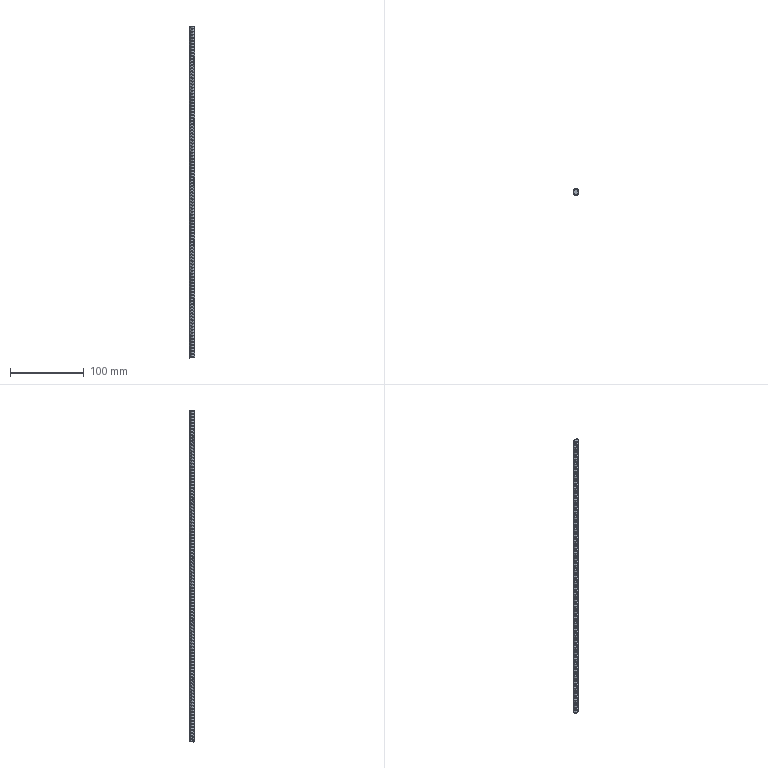Part | STEP file | Lead screw 1 | 1 solid | 230 faces | box 8 x 8 x 450 mm | volume 16512 mm3 | cylinder 227 | plane 2 | spline 1 | commonest cylinder face diameters 8 x227